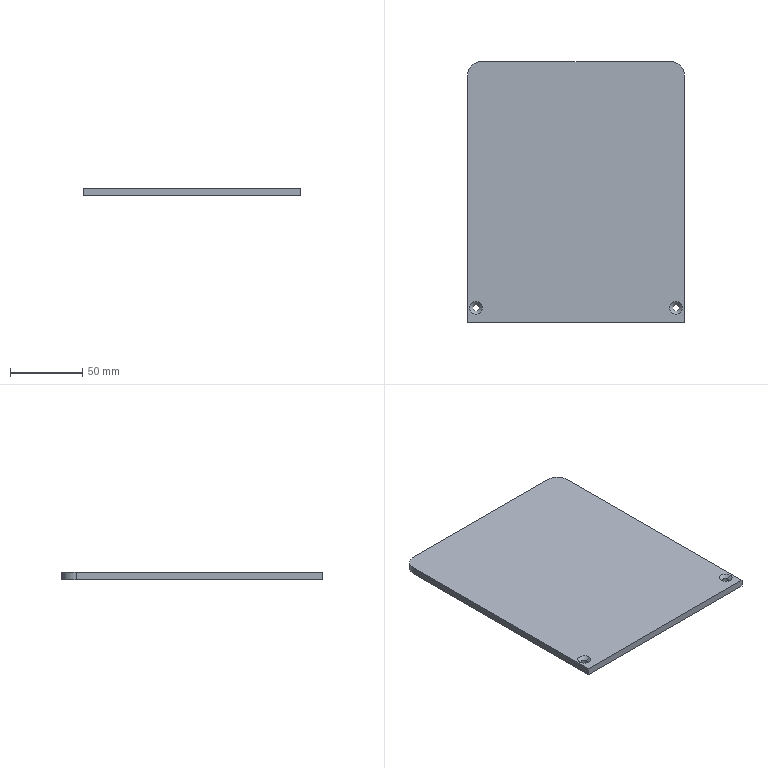Part | STEP file | ND25021-09-JDKM-008-SL | 1 solid | 16 faces | box 150 x 180 x 5 mm | volume 134533 mm3 | cylinder 6 | plane 6 | cone 4 | commonest cylinder face diameters 4.5 x4 20 x2
STEP:
#1=CARTESIAN_POINT('',(0.,0.,0.));
#2=DIRECTION('',(0.,0.,1.));
#3=DIRECTION('',(1.,0.,0.));
#4=AXIS2_PLACEMENT_3D('',#1,#2,#3);
#5=CARTESIAN_POINT('',(71.25,-80.,0.27));
#6=VERTEX_POINT('',#5);
#7=CARTESIAN_POINT('',(73.48,-80.,2.5));
#8=VERTEX_POINT('',#7);
#9=CARTESIAN_POINT('',(73.48,-80.,2.5));
#10=DIRECTION('',(0.7071,0.,0.7071));
#11=VECTOR('',#10,1.);
#12=LINE('',#9,#11);
#13=CARTESIAN_POINT('',(69.,-80.,2.5));
#14=DIRECTION('',(0.,0.,1.));
#15=DIRECTION('',(1.,0.,0.));
#16=AXIS2_PLACEMENT_3D('',#13,#14,#15);
#17=CONICAL_SURFACE('',#16,4.48,0.7854);
#18=CARTESIAN_POINT('',(6.283,0.));
#19=DIRECTION('',(0.,1.));
#20=VECTOR('',#19,1.);
#21=LINE('',#18,#20);
#22=(GEOMETRIC_REPRESENTATION_CONTEXT(2)PARAMETRIC_REPRESENTATION_CONTEXT()REPRESENTATION_CONTEXT('',''));
#23=DEFINITIONAL_REPRESENTATION('',(#21),#22);
#24=PCURVE('',#17,#23);
#25=CARTESIAN_POINT('',(69.,-80.,2.5));
#26=DIRECTION('',(0.,0.,1.));
#27=DIRECTION('',(1.,0.,0.));
#28=AXIS2_PLACEMENT_3D('',#25,#26,#27);
#29=CONICAL_SURFACE('',#28,4.48,0.7854);
#30=CARTESIAN_POINT('',(0.,0.));
#31=DIRECTION('',(0.,1.));
#32=VECTOR('',#31,1.);
#33=LINE('',#30,#32);
#34=(GEOMETRIC_REPRESENTATION_CONTEXT(2)PARAMETRIC_REPRESENTATION_CONTEXT()REPRESENTATION_CONTEXT('',''));
#35=DEFINITIONAL_REPRESENTATION('',(#33),#34);
#36=PCURVE('',#29,#35);
#37=SURFACE_CURVE('',#12,(#24,#36),.PCURVE_S1.);
#38=EDGE_CURVE('',#6,#8,#37,.T.);
#39=ORIENTED_EDGE('',*,*,#38,.T.);
#40=CARTESIAN_POINT('',(64.52,-80.,2.5));
#41=VERTEX_POINT('',#40);
#42=CARTESIAN_POINT('',(69.,-80.,2.5));
#43=DIRECTION('',(0.,0.,1.));
#44=DIRECTION('',(1.,0.,0.));
#45=AXIS2_PLACEMENT_3D('',#42,#43,#44);
#46=CIRCLE('',#45,4.48);
#47=CARTESIAN_POINT('',(0.,0.));
#48=DIRECTION('',(1.,0.));
#49=VECTOR('',#48,1.);
#50=LINE('',#47,#49);
#51=(GEOMETRIC_REPRESENTATION_CONTEXT(2)PARAMETRIC_REPRESENTATION_CONTEXT()REPRESENTATION_CONTEXT('',''));
#52=DEFINITIONAL_REPRESENTATION('',(#50),#51);
#53=PCURVE('',#17,#52);
#54=CARTESIAN_POINT('',(0.,0.,2.5));
#55=DIRECTION('',(0.,0.,1.));
#56=DIRECTION('',(1.,0.,0.));
#57=AXIS2_PLACEMENT_3D('',#54,#55,#56);
#58=PLANE('',#57);
#59=CARTESIAN_POINT('',(69.,-80.));
#60=DIRECTION('',(1.,0.));
#61=AXIS2_PLACEMENT_2D('',#59,#60);
#62=CIRCLE('',#61,4.48);
#63=(GEOMETRIC_REPRESENTATION_CONTEXT(2)PARAMETRIC_REPRESENTATION_CONTEXT()REPRESENTATION_CONTEXT('',''));
#64=DEFINITIONAL_REPRESENTATION('',(#62),#63);
#65=PCURVE('',#58,#64);
#66=SURFACE_CURVE('',#46,(#53,#65),.PCURVE_S1.);
#67=EDGE_CURVE('',#41,#8,#66,.T.);
#68=ORIENTED_EDGE('',*,*,#67,.F.);
#69=CARTESIAN_POINT('',(66.75,-80.,0.27));
#70=VERTEX_POINT('',#69);
#71=CARTESIAN_POINT('',(64.52,-80.,2.5));
#72=DIRECTION('',(-0.7071,0.,0.7071));
#73=VECTOR('',#72,1.);
#74=LINE('',#71,#73);
#75=CARTESIAN_POINT('',(3.142,0.));
#76=DIRECTION('',(0.,1.));
#77=VECTOR('',#76,1.);
#78=LINE('',#75,#77);
#79=(GEOMETRIC_REPRESENTATION_CONTEXT(2)PARAMETRIC_REPRESENTATION_CONTEXT()REPRESENTATION_CONTEXT('',''));
#80=DEFINITIONAL_REPRESENTATION('',(#78),#79);
#81=PCURVE('',#17,#80);
#82=CARTESIAN_POINT('',(3.142,0.));
#83=DIRECTION('',(0.,1.));
#84=VECTOR('',#83,1.);
#85=LINE('',#82,#84);
#86=(GEOMETRIC_REPRESENTATION_CONTEXT(2)PARAMETRIC_REPRESENTATION_CONTEXT()REPRESENTATION_CONTEXT('',''));
#87=DEFINITIONAL_REPRESENTATION('',(#85),#86);
#88=PCURVE('',#29,#87);
#89=SURFACE_CURVE('',#74,(#81,#88),.PCURVE_S1.);
#90=EDGE_CURVE('',#70,#41,#89,.T.);
#91=ORIENTED_EDGE('',*,*,#90,.F.);
#92=CARTESIAN_POINT('',(69.,-80.,0.27));
#93=DIRECTION('',(0.,0.,1.));
#94=DIRECTION('',(1.,0.,0.));
#95=AXIS2_PLACEMENT_3D('',#92,#93,#94);
#96=CIRCLE('',#95,2.25);
#97=CARTESIAN_POINT('',(0.,-2.23));
#98=DIRECTION('',(1.,0.));
#99=VECTOR('',#98,1.);
#100=LINE('',#97,#99);
#101=(GEOMETRIC_REPRESENTATION_CONTEXT(2)PARAMETRIC_REPRESENTATION_CONTEXT()REPRESENTATION_CONTEXT('',''));
#102=DEFINITIONAL_REPRESENTATION('',(#100),#101);
#103=PCURVE('',#17,#102);
#104=CARTESIAN_POINT('',(69.,-80.,2.5));
#105=DIRECTION('',(0.,0.,1.));
#106=DIRECTION('',(1.,0.,0.));
#107=AXIS2_PLACEMENT_3D('',#104,#105,#106);
#108=CYLINDRICAL_SURFACE('',#107,2.25);
#109=CARTESIAN_POINT('',(0.,-2.23));
#110=DIRECTION('',(1.,0.));
#111=VECTOR('',#110,1.);
#112=LINE('',#109,#111);
#113=(GEOMETRIC_REPRESENTATION_CONTEXT(2)PARAMETRIC_REPRESENTATION_CONTEXT()REPRESENTATION_CONTEXT('',''));
#114=DEFINITIONAL_REPRESENTATION('',(#112),#113);
#115=PCURVE('',#108,#114);
#116=SURFACE_CURVE('',#96,(#103,#115),.PCURVE_S1.);
#117=EDGE_CURVE('',#70,#6,#116,.T.);
#118=ORIENTED_EDGE('',*,*,#117,.T.);
#119=EDGE_LOOP('',(#39,#68,#91,#118));
#120=FACE_BOUND('',#119,.F.);
#121=ADVANCED_FACE('',(#120),#17,.F.);
#122=CARTESIAN_POINT('',(71.25,-80.,-2.5));
#123=VERTEX_POINT('',#122);
#124=CARTESIAN_POINT('',(71.25,-80.,2.5));
#125=DIRECTION('',(0.,0.,1.));
#126=VECTOR('',#125,1.);
#127=LINE('',#124,#126);
#128=CARTESIAN_POINT('',(6.283,0.));
#129=DIRECTION('',(0.,1.));
#130=VECTOR('',#129,1.);
#131=LINE('',#128,#130);
#132=(GEOMETRIC_REPRESENTATION_CONTEXT(2)PARAMETRIC_REPRESENTATION_CONTEXT()REPRESENTATION_CONTEXT('',''));
#133=DEFINITIONAL_REPRESENTATION('',(#131),#132);
#134=PCURVE('',#108,#133);
#135=CARTESIAN_POINT('',(69.,-80.,2.5));
#136=DIRECTION('',(0.,0.,1.));
#137=DIRECTION('',(1.,0.,0.));
#138=AXIS2_PLACEMENT_3D('',#135,#136,#137);
#139=CYLINDRICAL_SURFACE('',#138,2.25);
#140=CARTESIAN_POINT('',(0.,0.));
#141=DIRECTION('',(0.,1.));
#142=VECTOR('',#141,1.);
#143=LINE('',#140,#142);
#144=(GEOMETRIC_REPRESENTATION_CONTEXT(2)PARAMETRIC_REPRESENTATION_CONTEXT()REPRESENTATION_CONTEXT('',''));
#145=DEFINITIONAL_REPRESENTATION('',(#143),#144);
#146=PCURVE('',#139,#145);
#147=SURFACE_CURVE('',#127,(#134,#146),.PCURVE_S1.);
#148=EDGE_CURVE('',#123,#6,#147,.T.);
#149=ORIENTED_EDGE('',*,*,#148,.T.);
#150=ORIENTED_EDGE('',*,*,#117,.F.);
#151=CARTESIAN_POINT('',(66.75,-80.,-2.5));
#152=VERTEX_POINT('',#151);
#153=CARTESIAN_POINT('',(66.75,-80.,2.5));
#154=DIRECTION('',(0.,0.,1.));
#155=VECTOR('',#154,1.);
#156=LINE('',#153,#155);
#157=CARTESIAN_POINT('',(3.142,0.));
#158=DIRECTION('',(0.,1.));
#159=VECTOR('',#158,1.);
#160=LINE('',#157,#159);
#161=(GEOMETRIC_REPRESENTATION_CONTEXT(2)PARAMETRIC_REPRESENTATION_CONTEXT()REPRESENTATION_CONTEXT('',''));
#162=DEFINITIONAL_REPRESENTATION('',(#160),#161);
#163=PCURVE('',#108,#162);
#164=CARTESIAN_POINT('',(3.142,0.));
#165=DIRECTION('',(0.,1.));
#166=VECTOR('',#165,1.);
#167=LINE('',#164,#166);
#168=(GEOMETRIC_REPRESENTATION_CONTEXT(2)PARAMETRIC_REPRESENTATION_CONTEXT()REPRESENTATION_CONTEXT('',''));
#169=DEFINITIONAL_REPRESENTATION('',(#167),#168);
#170=PCURVE('',#139,#169);
#171=SURFACE_CURVE('',#156,(#163,#170),.PCURVE_S1.);
#172=EDGE_CURVE('',#152,#70,#171,.T.);
#173=ORIENTED_EDGE('',*,*,#172,.F.);
#174=CARTESIAN_POINT('',(69.,-80.,-2.5));
#175=DIRECTION('',(0.,0.,1.));
#176=DIRECTION('',(1.,0.,0.));
#177=AXIS2_PLACEMENT_3D('',#174,#175,#176);
#178=CIRCLE('',#177,2.25);
#179=CARTESIAN_POINT('',(0.,-5.));
#180=DIRECTION('',(1.,0.));
#181=VECTOR('',#180,1.);
#182=LINE('',#179,#181);
#183=(GEOMETRIC_REPRESENTATION_CONTEXT(2)PARAMETRIC_REPRESENTATION_CONTEXT()REPRESENTATION_CONTEXT('',''));
#184=DEFINITIONAL_REPRESENTATION('',(#182),#183);
#185=PCURVE('',#108,#184);
#186=CARTESIAN_POINT('',(0.,0.,-2.5));
#187=DIRECTION('',(0.,0.,1.));
#188=DIRECTION('',(1.,0.,0.));
#189=AXIS2_PLACEMENT_3D('',#186,#187,#188);
#190=PLANE('',#189);
#191=CARTESIAN_POINT('',(69.,-80.));
#192=DIRECTION('',(1.,0.));
#193=AXIS2_PLACEMENT_2D('',#191,#192);
#194=CIRCLE('',#193,2.25);
#195=(GEOMETRIC_REPRESENTATION_CONTEXT(2)PARAMETRIC_REPRESENTATION_CONTEXT()REPRESENTATION_CONTEXT('',''));
#196=DEFINITIONAL_REPRESENTATION('',(#194),#195);
#197=PCURVE('',#190,#196);
#198=SURFACE_CURVE('',#178,(#185,#197),.PCURVE_S1.);
#199=EDGE_CURVE('',#152,#123,#198,.T.);
#200=ORIENTED_EDGE('',*,*,#199,.T.);
#201=EDGE_LOOP('',(#149,#150,#173,#200));
#202=FACE_BOUND('',#201,.F.);
#203=ADVANCED_FACE('',(#202),#108,.F.);
#204=CARTESIAN_POINT('',(-66.75,-80.,0.27));
#205=VERTEX_POINT('',#204);
#206=CARTESIAN_POINT('',(-64.52,-80.,2.5));
#207=VERTEX_POINT('',#206);
#208=CARTESIAN_POINT('',(-64.52,-80.,2.5));
#209=DIRECTION('',(0.7071,0.,0.7071));
#210=VECTOR('',#209,1.);
#211=LINE('',#208,#210);
#212=CARTESIAN_POINT('',(-69.,-80.,2.5));
#213=DIRECTION('',(0.,0.,1.));
#214=DIRECTION('',(1.,0.,0.));
#215=AXIS2_PLACEMENT_3D('',#212,#213,#214);
#216=CONICAL_SURFACE('',#215,4.48,0.7854);
#217=CARTESIAN_POINT('',(6.283,0.));
#218=DIRECTION('',(0.,1.));
#219=VECTOR('',#218,1.);
#220=LINE('',#217,#219);
#221=(GEOMETRIC_REPRESENTATION_CONTEXT(2)PARAMETRIC_REPRESENTATION_CONTEXT()REPRESENTATION_CONTEXT('',''));
#222=DEFINITIONAL_REPRESENTATION('',(#220),#221);
#223=PCURVE('',#216,#222);
#224=CARTESIAN_POINT('',(-69.,-80.,2.5));
#225=DIRECTION('',(0.,0.,1.));
#226=DIRECTION('',(1.,0.,0.));
#227=AXIS2_PLACEMENT_3D('',#224,#225,#226);
#228=CONICAL_SURFACE('',#227,4.48,0.7854);
#229=CARTESIAN_POINT('',(0.,0.));
#230=DIRECTION('',(0.,1.));
#231=VECTOR('',#230,1.);
#232=LINE('',#229,#231);
#233=(GEOMETRIC_REPRESENTATION_CONTEXT(2)PARAMETRIC_REPRESENTATION_CONTEXT()REPRESENTATION_CONTEXT('',''));
#234=DEFINITIONAL_REPRESENTATION('',(#232),#233);
#235=PCURVE('',#228,#234);
#236=SURFACE_CURVE('',#211,(#223,#235),.PCURVE_S1.);
#237=EDGE_CURVE('',#205,#207,#236,.T.);
#238=ORIENTED_EDGE('',*,*,#237,.T.);
#239=CARTESIAN_POINT('',(-73.48,-80.,2.5));
#240=VERTEX_POINT('',#239);
#241=CARTESIAN_POINT('',(-69.,-80.,2.5));
#242=DIRECTION('',(0.,0.,1.));
#243=DIRECTION('',(1.,0.,0.));
#244=AXIS2_PLACEMENT_3D('',#241,#242,#243);
#245=CIRCLE('',#244,4.48);
#246=CARTESIAN_POINT('',(0.,0.));
#247=DIRECTION('',(1.,0.));
#248=VECTOR('',#247,1.);
#249=LINE('',#246,#248);
#250=(GEOMETRIC_REPRESENTATION_CONTEXT(2)PARAMETRIC_REPRESENTATION_CONTEXT()REPRESENTATION_CONTEXT('',''));
#251=DEFINITIONAL_REPRESENTATION('',(#249),#250);
#252=PCURVE('',#216,#251);
#253=CARTESIAN_POINT('',(-69.,-80.));
#254=DIRECTION('',(1.,0.));
#255=AXIS2_PLACEMENT_2D('',#253,#254);
#256=CIRCLE('',#255,4.48);
#257=(GEOMETRIC_REPRESENTATION_CONTEXT(2)PARAMETRIC_REPRESENTATION_CONTEXT()REPRESENTATION_CONTEXT('',''));
#258=DEFINITIONAL_REPRESENTATION('',(#256),#257);
#259=PCURVE('',#58,#258);
#260=SURFACE_CURVE('',#245,(#252,#259),.PCURVE_S1.);
#261=EDGE_CURVE('',#240,#207,#260,.T.);
#262=ORIENTED_EDGE('',*,*,#261,.F.);
#263=CARTESIAN_POINT('',(-71.25,-80.,0.27));
#264=VERTEX_POINT('',#263);
#265=CARTESIAN_POINT('',(-73.48,-80.,2.5));
#266=DIRECTION('',(-0.7071,0.,0.7071));
#267=VECTOR('',#266,1.);
#268=LINE('',#265,#267);
#269=CARTESIAN_POINT('',(3.142,0.));
#270=DIRECTION('',(0.,1.));
#271=VECTOR('',#270,1.);
#272=LINE('',#269,#271);
#273=(GEOMETRIC_REPRESENTATION_CONTEXT(2)PARAMETRIC_REPRESENTATION_CONTEXT()REPRESENTATION_CONTEXT('',''));
#274=DEFINITIONAL_REPRESENTATION('',(#272),#273);
#275=PCURVE('',#216,#274);
#276=CARTESIAN_POINT('',(3.142,0.));
#277=DIRECTION('',(0.,1.));
#278=VECTOR('',#277,1.);
#279=LINE('',#276,#278);
#280=(GEOMETRIC_REPRESENTATION_CONTEXT(2)PARAMETRIC_REPRESENTATION_CONTEXT()REPRESENTATION_CONTEXT('',''));
#281=DEFINITIONAL_REPRESENTATION('',(#279),#280);
#282=PCURVE('',#228,#281);
#283=SURFACE_CURVE('',#268,(#275,#282),.PCURVE_S1.);
#284=EDGE_CURVE('',#264,#240,#283,.T.);
#285=ORIENTED_EDGE('',*,*,#284,.F.);
#286=CARTESIAN_POINT('',(-69.,-80.,0.27));
#287=DIRECTION('',(0.,0.,1.));
#288=DIRECTION('',(1.,0.,0.));
#289=AXIS2_PLACEMENT_3D('',#286,#287,#288);
#290=CIRCLE('',#289,2.25);
#291=CARTESIAN_POINT('',(0.,-2.23));
#292=DIRECTION('',(1.,0.));
#293=VECTOR('',#292,1.);
#294=LINE('',#291,#293);
#295=(GEOMETRIC_REPRESENTATION_CONTEXT(2)PARAMETRIC_REPRESENTATION_CONTEXT()REPRESENTATION_CONTEXT('',''));
#296=DEFINITIONAL_REPRESENTATION('',(#294),#295);
#297=PCURVE('',#216,#296);
#298=CARTESIAN_POINT('',(-69.,-80.,2.5));
#299=DIRECTION('',(0.,0.,1.));
#300=DIRECTION('',(1.,0.,0.));
#301=AXIS2_PLACEMENT_3D('',#298,#299,#300);
#302=CYLINDRICAL_SURFACE('',#301,2.25);
#303=CARTESIAN_POINT('',(0.,-2.23));
#304=DIRECTION('',(1.,0.));
#305=VECTOR('',#304,1.);
#306=LINE('',#303,#305);
#307=(GEOMETRIC_REPRESENTATION_CONTEXT(2)PARAMETRIC_REPRESENTATION_CONTEXT()REPRESENTATION_CONTEXT('',''));
#308=DEFINITIONAL_REPRESENTATION('',(#306),#307);
#309=PCURVE('',#302,#308);
#310=SURFACE_CURVE('',#290,(#297,#309),.PCURVE_S1.);
#311=EDGE_CURVE('',#264,#205,#310,.T.);
#312=ORIENTED_EDGE('',*,*,#311,.T.);
#313=EDGE_LOOP('',(#238,#262,#285,#312));
#314=FACE_BOUND('',#313,.F.);
#315=ADVANCED_FACE('',(#314),#216,.F.);
#316=CARTESIAN_POINT('',(-66.75,-80.,-2.5));
#317=VERTEX_POINT('',#316);
#318=CARTESIAN_POINT('',(-66.75,-80.,2.5));
#319=DIRECTION('',(0.,0.,1.));
#320=VECTOR('',#319,1.);
#321=LINE('',#318,#320);
#322=CARTESIAN_POINT('',(6.283,0.));
#323=DIRECTION('',(0.,1.));
#324=VECTOR('',#323,1.);
#325=LINE('',#322,#324);
#326=(GEOMETRIC_REPRESENTATION_CONTEXT(2)PARAMETRIC_REPRESENTATION_CONTEXT()REPRESENTATION_CONTEXT('',''));
#327=DEFINITIONAL_REPRESENTATION('',(#325),#326);
#328=PCURVE('',#302,#327);
#329=CARTESIAN_POINT('',(-69.,-80.,2.5));
#330=DIRECTION('',(0.,0.,1.));
#331=DIRECTION('',(1.,0.,0.));
#332=AXIS2_PLACEMENT_3D('',#329,#330,#331);
#333=CYLINDRICAL_SURFACE('',#332,2.25);
#334=CARTESIAN_POINT('',(0.,0.));
#335=DIRECTION('',(0.,1.));
#336=VECTOR('',#335,1.);
#337=LINE('',#334,#336);
#338=(GEOMETRIC_REPRESENTATION_CONTEXT(2)PARAMETRIC_REPRESENTATION_CONTEXT()REPRESENTATION_CONTEXT('',''));
#339=DEFINITIONAL_REPRESENTATION('',(#337),#338);
#340=PCURVE('',#333,#339);
#341=SURFACE_CURVE('',#321,(#328,#340),.PCURVE_S1.);
#342=EDGE_CURVE('',#317,#205,#341,.T.);
#343=ORIENTED_EDGE('',*,*,#342,.T.);
#344=ORIENTED_EDGE('',*,*,#311,.F.);
#345=CARTESIAN_POINT('',(-71.25,-80.,-2.5));
#346=VERTEX_POINT('',#345);
#347=CARTESIAN_POINT('',(-71.25,-80.,2.5));
#348=DIRECTION('',(0.,0.,1.));
#349=VECTOR('',#348,1.);
#350=LINE('',#347,#349);
#351=CARTESIAN_POINT('',(3.142,0.));
#352=DIRECTION('',(0.,1.));
#353=VECTOR('',#352,1.);
#354=LINE('',#351,#353);
#355=(GEOMETRIC_REPRESENTATION_CONTEXT(2)PARAMETRIC_REPRESENTATION_CONTEXT()REPRESENTATION_CONTEXT('',''));
#356=DEFINITIONAL_REPRESENTATION('',(#354),#355);
#357=PCURVE('',#302,#356);
#358=CARTESIAN_POINT('',(3.142,0.));
#359=DIRECTION('',(0.,1.));
#360=VECTOR('',#359,1.);
#361=LINE('',#358,#360);
#362=(GEOMETRIC_REPRESENTATION_CONTEXT(2)PARAMETRIC_REPRESENTATION_CONTEXT()REPRESENTATION_CONTEXT('',''));
#363=DEFINITIONAL_REPRESENTATION('',(#361),#362);
#364=PCURVE('',#333,#363);
#365=SURFACE_CURVE('',#350,(#357,#364),.PCURVE_S1.);
#366=EDGE_CURVE('',#346,#264,#365,.T.);
#367=ORIENTED_EDGE('',*,*,#366,.F.);
#368=CARTESIAN_POINT('',(-69.,-80.,-2.5));
#369=DIRECTION('',(0.,0.,1.));
#370=DIRECTION('',(1.,0.,0.));
#371=AXIS2_PLACEMENT_3D('',#368,#369,#370);
#372=CIRCLE('',#371,2.25);
#373=CARTESIAN_POINT('',(0.,-5.));
#374=DIRECTION('',(1.,0.));
#375=VECTOR('',#374,1.);
#376=LINE('',#373,#375);
#377=(GEOMETRIC_REPRESENTATION_CONTEXT(2)PARAMETRIC_REPRESENTATION_CONTEXT()REPRESENTATION_CONTEXT('',''));
#378=DEFINITIONAL_REPRESENTATION('',(#376),#377);
#379=PCURVE('',#302,#378);
#380=CARTESIAN_POINT('',(-69.,-80.));
#381=DIRECTION('',(1.,0.));
#382=AXIS2_PLACEMENT_2D('',#380,#381);
#383=CIRCLE('',#382,2.25);
#384=(GEOMETRIC_REPRESENTATION_CONTEXT(2)PARAMETRIC_REPRESENTATION_CONTEXT()REPRESENTATION_CONTEXT('',''));
#385=DEFINITIONAL_REPRESENTATION('',(#383),#384);
#386=PCURVE('',#190,#385);
#387=SURFACE_CURVE('',#372,(#379,#386),.PCURVE_S1.);
#388=EDGE_CURVE('',#346,#317,#387,.T.);
#389=ORIENTED_EDGE('',*,*,#388,.T.);
#390=EDGE_LOOP('',(#343,#344,#367,#389));
#391=FACE_BOUND('',#390,.F.);
#392=ADVANCED_FACE('',(#391),#302,.F.);
#393=CARTESIAN_POINT('',(75.,-90.,-2.5));
#394=VERTEX_POINT('',#393);
#395=CARTESIAN_POINT('',(75.,80.,-2.5));
#396=VERTEX_POINT('',#395);
#397=CARTESIAN_POINT('',(75.,90.,-2.5));
#398=DIRECTION('',(0.,1.,0.));
#399=VECTOR('',#398,1.);
#400=LINE('',#397,#399);
#401=CARTESIAN_POINT('',(75.,90.,2.5));
#402=DIRECTION('',(-1.,0.,0.));
#403=DIRECTION('',(0.,-1.,0.));
#404=AXIS2_PLACEMENT_3D('',#401,#402,#403);
#405=PLANE('',#404);
#406=CARTESIAN_POINT('',(0.,-5.));
#407=DIRECTION('',(-1.,0.));
#408=VECTOR('',#407,1.);
#409=LINE('',#406,#408);
#410=(GEOMETRIC_REPRESENTATION_CONTEXT(2)PARAMETRIC_REPRESENTATION_CONTEXT()REPRESENTATION_CONTEXT('',''));
#411=DEFINITIONAL_REPRESENTATION('',(#409),#410);
#412=PCURVE('',#405,#411);
#413=CARTESIAN_POINT('',(75.,90.));
#414=DIRECTION('',(0.,1.));
#415=VECTOR('',#414,1.);
#416=LINE('',#413,#415);
#417=(GEOMETRIC_REPRESENTATION_CONTEXT(2)PARAMETRIC_REPRESENTATION_CONTEXT()REPRESENTATION_CONTEXT('',''));
#418=DEFINITIONAL_REPRESENTATION('',(#416),#417);
#419=PCURVE('',#190,#418);
#420=SURFACE_CURVE('',#400,(#412,#419),.PCURVE_S1.);
#421=EDGE_CURVE('',#394,#396,#420,.T.);
#422=ORIENTED_EDGE('',*,*,#421,.T.);
#423=CARTESIAN_POINT('',(75.,80.,2.5));
#424=VERTEX_POINT('',#423);
#425=CARTESIAN_POINT('',(75.,80.,2.5));
#426=DIRECTION('',(0.,0.,1.));
#427=VECTOR('',#426,1.);
#428=LINE('',#425,#427);
#429=CARTESIAN_POINT('',(10.,0.));
#430=DIRECTION('',(0.,1.));
#431=VECTOR('',#430,1.);
#432=LINE('',#429,#431);
#433=(GEOMETRIC_REPRESENTATION_CONTEXT(2)PARAMETRIC_REPRESENTATION_CONTEXT()REPRESENTATION_CONTEXT('',''));
#434=DEFINITIONAL_REPRESENTATION('',(#432),#433);
#435=PCURVE('',#405,#434);
#436=CARTESIAN_POINT('',(65.,80.,2.5));
#437=DIRECTION('',(0.,0.,-1.));
#438=DIRECTION('',(-1.,0.,0.));
#439=AXIS2_PLACEMENT_3D('',#436,#437,#438);
#440=CYLINDRICAL_SURFACE('',#439,10.);
#441=CARTESIAN_POINT('',(3.142,0.));
#442=DIRECTION('',(0.,-1.));
#443=VECTOR('',#442,1.);
#444=LINE('',#441,#443);
#445=(GEOMETRIC_REPRESENTATION_CONTEXT(2)PARAMETRIC_REPRESENTATION_CONTEXT()REPRESENTATION_CONTEXT('',''));
#446=DEFINITIONAL_REPRESENTATION('',(#444),#445);
#447=PCURVE('',#440,#446);
#448=SURFACE_CURVE('',#428,(#435,#447),.PCURVE_S1.);
#449=EDGE_CURVE('',#396,#424,#448,.T.);
#450=ORIENTED_EDGE('',*,*,#449,.T.);
#451=CARTESIAN_POINT('',(75.,-90.,2.5));
#452=VERTEX_POINT('',#451);
#453=CARTESIAN_POINT('',(75.,90.,2.5));
#454=DIRECTION('',(0.,1.,0.));
#455=VECTOR('',#454,1.);
#456=LINE('',#453,#455);
#457=CARTESIAN_POINT('',(0.,0.));
#458=DIRECTION('',(-1.,0.));
#459=VECTOR('',#458,1.);
#460=LINE('',#457,#459);
#461=(GEOMETRIC_REPRESENTATION_CONTEXT(2)PARAMETRIC_REPRESENTATION_CONTEXT()REPRESENTATION_CONTEXT('',''));
#462=DEFINITIONAL_REPRESENTATION('',(#460),#461);
#463=PCURVE('',#405,#462);
#464=CARTESIAN_POINT('',(75.,90.));
#465=DIRECTION('',(0.,1.));
#466=VECTOR('',#465,1.);
#467=LINE('',#464,#466);
#468=(GEOMETRIC_REPRESENTATION_CONTEXT(2)PARAMETRIC_REPRESENTATION_CONTEXT()REPRESENTATION_CONTEXT('',''));
#469=DEFINITIONAL_REPRESENTATION('',(#467),#468);
#470=PCURVE('',#58,#469);
#471=SURFACE_CURVE('',#456,(#463,#470),.PCURVE_S1.);
#472=EDGE_CURVE('',#452,#424,#471,.T.);
#473=ORIENTED_EDGE('',*,*,#472,.F.);
#474=CARTESIAN_POINT('',(75.,-90.,2.5));
#475=DIRECTION('',(0.,0.,-1.));
#476=VECTOR('',#475,1.);
#477=LINE('',#474,#476);
#478=CARTESIAN_POINT('',(180.,0.));
#479=DIRECTION('',(0.,-1.));
#480=VECTOR('',#479,1.);
#481=LINE('',#478,#480);
#482=(GEOMETRIC_REPRESENTATION_CONTEXT(2)PARAMETRIC_REPRESENTATION_CONTEXT()REPRESENTATION_CONTEXT('',''));
#483=DEFINITIONAL_REPRESENTATION('',(#481),#482);
#484=PCURVE('',#405,#483);
#485=CARTESIAN_POINT('',(-75.,-90.,2.5));
#486=DIRECTION('',(0.,1.,0.));
#487=DIRECTION('',(0.,0.,1.));
#488=AXIS2_PLACEMENT_3D('',#485,#486,#487);
#489=PLANE('',#488);
#490=CARTESIAN_POINT('',(0.,150.));
#491=DIRECTION('',(-1.,0.));
#492=VECTOR('',#491,1.);
#493=LINE('',#490,#492);
#494=(GEOMETRIC_REPRESENTATION_CONTEXT(2)PARAMETRIC_REPRESENTATION_CONTEXT()REPRESENTATION_CONTEXT('',''));
#495=DEFINITIONAL_REPRESENTATION('',(#493),#494);
#496=PCURVE('',#489,#495);
#497=SURFACE_CURVE('',#477,(#484,#496),.PCURVE_S1.);
#498=EDGE_CURVE('',#452,#394,#497,.T.);
#499=ORIENTED_EDGE('',*,*,#498,.T.);
#500=EDGE_LOOP('',(#422,#450,#473,#499));
#501=FACE_BOUND('',#500,.T.);
#502=ADVANCED_FACE('',(#501),#405,.F.);
#503=CARTESIAN_POINT('',(65.,90.,-2.5));
#504=VERTEX_POINT('',#503);
#505=CARTESIAN_POINT('',(-65.,90.,-2.5));
#506=VERTEX_POINT('',#505);
#507=CARTESIAN_POINT('',(-75.,90.,-2.5));
#508=DIRECTION('',(-1.,0.,0.));
#509=VECTOR('',#508,1.);
#510=LINE('',#507,#509);
#511=CARTESIAN_POINT('',(-75.,90.,2.5));
#512=DIRECTION('',(0.,-1.,0.));
#513=DIRECTION('',(0.,0.,-1.));
#514=AXIS2_PLACEMENT_3D('',#511,#512,#513);
#515=PLANE('',#514);
#516=CARTESIAN_POINT('',(5.,0.));
#517=DIRECTION('',(0.,-1.));
#518=VECTOR('',#517,1.);
#519=LINE('',#516,#518);
#520=(GEOMETRIC_REPRESENTATION_CONTEXT(2)PARAMETRIC_REPRESENTATION_CONTEXT()REPRESENTATION_CONTEXT('',''));
#521=DEFINITIONAL_REPRESENTATION('',(#519),#520);
#522=PCURVE('',#515,#521);
#523=CARTESIAN_POINT('',(-75.,90.));
#524=DIRECTION('',(-1.,0.));
#525=VECTOR('',#524,1.);
#526=LINE('',#523,#525);
#527=(GEOMETRIC_REPRESENTATION_CONTEXT(2)PARAMETRIC_REPRESENTATION_CONTEXT()REPRESENTATION_CONTEXT('',''));
#528=DEFINITIONAL_REPRESENTATION('',(#526),#527);
#529=PCURVE('',#190,#528);
#530=SURFACE_CURVE('',#510,(#522,#529),.PCURVE_S1.);
#531=EDGE_CURVE('',#504,#506,#530,.T.);
#532=ORIENTED_EDGE('',*,*,#531,.T.);
#533=CARTESIAN_POINT('',(-65.,90.,2.5));
#534=VERTEX_POINT('',#533);
#535=CARTESIAN_POINT('',(-65.,90.,2.5));
#536=DIRECTION('',(0.,0.,1.));
#537=VECTOR('',#536,1.);
#538=LINE('',#535,#537);
#539=CARTESIAN_POINT('',(0.,10.));
#540=DIRECTION('',(-1.,0.));
#541=VECTOR('',#540,1.);
#542=LINE('',#539,#541);
#543=(GEOMETRIC_REPRESENTATION_CONTEXT(2)PARAMETRIC_REPRESENTATION_CONTEXT()REPRESENTATION_CONTEXT('',''));
#544=DEFINITIONAL_REPRESENTATION('',(#542),#543);
#545=PCURVE('',#515,#544);
#546=CARTESIAN_POINT('',(-65.,80.,2.5));
#547=DIRECTION('',(0.,0.,-1.));
#548=DIRECTION('',(-1.,0.,0.));
#549=AXIS2_PLACEMENT_3D('',#546,#547,#548);
#550=CYLINDRICAL_SURFACE('',#549,10.);
#551=CARTESIAN_POINT('',(1.571,0.));
#552=DIRECTION('',(0.,-1.));
#553=VECTOR('',#552,1.);
#554=LINE('',#551,#553);
#555=(GEOMETRIC_REPRESENTATION_CONTEXT(2)PARAMETRIC_REPRESENTATION_CONTEXT()REPRESENTATION_CONTEXT('',''));
#556=DEFINITIONAL_REPRESENTATION('',(#554),#555);
#557=PCURVE('',#550,#556);
#558=SURFACE_CURVE('',#538,(#545,#557),.PCURVE_S1.);
#559=EDGE_CURVE('',#506,#534,#558,.T.);
#560=ORIENTED_EDGE('',*,*,#559,.T.);
#561=CARTESIAN_POINT('',(65.,90.,2.5));
#562=VERTEX_POINT('',#561);
#563=CARTESIAN_POINT('',(-75.,90.,2.5));
#564=DIRECTION('',(-1.,0.,0.));
#565=VECTOR('',#564,1.);
#566=LINE('',#563,#565);
#567=CARTESIAN_POINT('',(0.,0.));
#568=DIRECTION('',(0.,-1.));
#569=VECTOR('',#568,1.);
#570=LINE('',#567,#569);
#571=(GEOMETRIC_REPRESENTATION_CONTEXT(2)PARAMETRIC_REPRESENTATION_CONTEXT()REPRESENTATION_CONTEXT('',''));
#572=DEFINITIONAL_REPRESENTATION('',(#570),#571);
#573=PCURVE('',#515,#572);
#574=CARTESIAN_POINT('',(-75.,90.));
#575=DIRECTION('',(-1.,0.));
#576=VECTOR('',#575,1.);
#577=LINE('',#574,#576);
#578=(GEOMETRIC_REPRESENTATION_CONTEXT(2)PARAMETRIC_REPRESENTATION_CONTEXT()REPRESENTATION_CONTEXT('',''));
#579=DEFINITIONAL_REPRESENTATION('',(#577),#578);
#580=PCURVE('',#58,#579);
#581=SURFACE_CURVE('',#566,(#573,#580),.PCURVE_S1.);
#582=EDGE_CURVE('',#562,#534,#581,.T.);
#583=ORIENTED_EDGE('',*,*,#582,.F.);
#584=CARTESIAN_POINT('',(65.,90.,2.5));
#585=DIRECTION('',(0.,0.,-1.));
#586=VECTOR('',#585,1.);
#587=LINE('',#584,#586);
#588=CARTESIAN_POINT('',(0.,140.));
#589=DIRECTION('',(1.,0.));
#590=VECTOR('',#589,1.);
#591=LINE('',#588,#590);
#592=(GEOMETRIC_REPRESENTATION_CONTEXT(2)PARAMETRIC_REPRESENTATION_CONTEXT()REPRESENTATION_CONTEXT('',''));
#593=DEFINITIONAL_REPRESENTATION('',(#591),#592);
#594=PCURVE('',#515,#593);
#595=CARTESIAN_POINT('',(1.571,0.));
#596=DIRECTION('',(0.,1.));
#597=VECTOR('',#596,1.);
#598=LINE('',#595,#597);
#599=(GEOMETRIC_REPRESENTATION_CONTEXT(2)PARAMETRIC_REPRESENTATION_CONTEXT()REPRESENTATION_CONTEXT('',''));
#600=DEFINITIONAL_REPRESENTATION('',(#598),#599);
#601=PCURVE('',#440,#600);
#602=SURFACE_CURVE('',#587,(#594,#601),.PCURVE_S1.);
#603=EDGE_CURVE('',#562,#504,#602,.T.);
#604=ORIENTED_EDGE('',*,*,#603,.T.);
#605=EDGE_LOOP('',(#532,#560,#583,#604));
#606=FACE_BOUND('',#605,.T.);
#607=ADVANCED_FACE('',(#606),#515,.F.);
#608=CARTESIAN_POINT('',(-75.,80.,2.5));
#609=VERTEX_POINT('',#608);
#610=CARTESIAN_POINT('',(-75.,-90.,2.5));
#611=VERTEX_POINT('',#610);
#612=CARTESIAN_POINT('',(-75.,90.,2.5));
#613=DIRECTION('',(0.,-1.,0.));
#614=VECTOR('',#613,1.);
#615=LINE('',#612,#614);
#616=CARTESIAN_POINT('',(-75.,90.,2.5));
#617=DIRECTION('',(1.,0.,0.));
#618=DIRECTION('',(0.,1.,0.));
#619=AXIS2_PLACEMENT_3D('',#616,#617,#618);
#620=PLANE('',#619);
#621=CARTESIAN_POINT('',(0.,0.));
#622=DIRECTION('',(-1.,0.));
#623=VECTOR('',#622,1.);
#624=LINE('',#621,#623);
#625=(GEOMETRIC_REPRESENTATION_CONTEXT(2)PARAMETRIC_REPRESENTATION_CONTEXT()REPRESENTATION_CONTEXT('',''));
#626=DEFINITIONAL_REPRESENTATION('',(#624),#625);
#627=PCURVE('',#620,#626);
#628=CARTESIAN_POINT('',(-75.,90.));
#629=DIRECTION('',(0.,-1.));
#630=VECTOR('',#629,1.);
#631=LINE('',#628,#630);
#632=(GEOMETRIC_REPRESENTATION_CONTEXT(2)PARAMETRIC_REPRESENTATION_CONTEXT()REPRESENTATION_CONTEXT('',''));
#633=DEFINITIONAL_REPRESENTATION('',(#631),#632);
#634=PCURVE('',#58,#633);
#635=SURFACE_CURVE('',#615,(#627,#634),.PCURVE_S1.);
#636=EDGE_CURVE('',#609,#611,#635,.T.);
#637=ORIENTED_EDGE('',*,*,#636,.F.);
#638=CARTESIAN_POINT('',(-75.,80.,-2.5));
#639=VERTEX_POINT('',#638);
#640=CARTESIAN_POINT('',(-75.,80.,2.5));
#641=DIRECTION('',(0.,0.,-1.));
#642=VECTOR('',#641,1.);
#643=LINE('',#640,#642);
#644=CARTESIAN_POINT('',(-10.,0.));
#645=DIRECTION('',(0.,-1.));
#646=VECTOR('',#645,1.);
#647=LINE('',#644,#646);
#648=(GEOMETRIC_REPRESENTATION_CONTEXT(2)PARAMETRIC_REPRESENTATION_CONTEXT()REPRESENTATION_CONTEXT('',''));
#649=DEFINITIONAL_REPRESENTATION('',(#647),#648);
#650=PCURVE('',#620,#649);
#651=CARTESIAN_POINT('',(0.,0.));
#652=DIRECTION('',(0.,1.));
#653=VECTOR('',#652,1.);
#654=LINE('',#651,#653);
#655=(GEOMETRIC_REPRESENTATION_CONTEXT(2)PARAMETRIC_REPRESENTATION_CONTEXT()REPRESENTATION_CONTEXT('',''));
#656=DEFINITIONAL_REPRESENTATION('',(#654),#655);
#657=PCURVE('',#550,#656);
#658=SURFACE_CURVE('',#643,(#650,#657),.PCURVE_S1.);
#659=EDGE_CURVE('',#609,#639,#658,.T.);
#660=ORIENTED_EDGE('',*,*,#659,.T.);
#661=CARTESIAN_POINT('',(-75.,-90.,-2.5));
#662=VERTEX_POINT('',#661);
#663=CARTESIAN_POINT('',(-75.,90.,-2.5));
#664=DIRECTION('',(0.,-1.,0.));
#665=VECTOR('',#664,1.);
#666=LINE('',#663,#665);
#667=CARTESIAN_POINT('',(0.,-5.));
#668=DIRECTION('',(-1.,0.));
#669=VECTOR('',#668,1.);
#670=LINE('',#667,#669);
#671=(GEOMETRIC_REPRESENTATION_CONTEXT(2)PARAMETRIC_REPRESENTATION_CONTEXT()REPRESENTATION_CONTEXT('',''));
#672=DEFINITIONAL_REPRESENTATION('',(#670),#671);
#673=PCURVE('',#620,#672);
#674=CARTESIAN_POINT('',(-75.,90.));
#675=DIRECTION('',(0.,-1.));
#676=VECTOR('',#675,1.);
#677=LINE('',#674,#676);
#678=(GEOMETRIC_REPRESENTATION_CONTEXT(2)PARAMETRIC_REPRESENTATION_CONTEXT()REPRESENTATION_CONTEXT('',''));
#679=DEFINITIONAL_REPRESENTATION('',(#677),#678);
#680=PCURVE('',#190,#679);
#681=SURFACE_CURVE('',#666,(#673,#680),.PCURVE_S1.);
#682=EDGE_CURVE('',#639,#662,#681,.T.);
#683=ORIENTED_EDGE('',*,*,#682,.T.);
#684=CARTESIAN_POINT('',(-75.,-90.,2.5));
#685=DIRECTION('',(0.,0.,-1.));
#686=VECTOR('',#685,1.);
#687=LINE('',#684,#686);
#688=CARTESIAN_POINT('',(-180.,0.));
#689=DIRECTION('',(0.,-1.));
#690=VECTOR('',#689,1.);
#691=LINE('',#688,#690);
#692=(GEOMETRIC_REPRESENTATION_CONTEXT(2)PARAMETRIC_REPRESENTATION_CONTEXT()REPRESENTATION_CONTEXT('',''));
#693=DEFINITIONAL_REPRESENTATION('',(#691),#692);
#694=PCURVE('',#620,#693);
#695=CARTESIAN_POINT('',(0.,0.));
#696=DIRECTION('',(-1.,0.));
#697=VECTOR('',#696,1.);
#698=LINE('',#695,#697);
#699=(GEOMETRIC_REPRESENTATION_CONTEXT(2)PARAMETRIC_REPRESENTATION_CONTEXT()REPRESENTATION_CONTEXT('',''));
#700=DEFINITIONAL_REPRESENTATION('',(#698),#699);
#701=PCURVE('',#489,#700);
#702=SURFACE_CURVE('',#687,(#694,#701),.PCURVE_S1.);
#703=EDGE_CURVE('',#611,#662,#702,.T.);
#704=ORIENTED_EDGE('',*,*,#703,.F.);
#705=EDGE_LOOP('',(#637,#660,#683,#704));
#706=FACE_BOUND('',#705,.T.);
#707=ADVANCED_FACE('',(#706),#620,.F.);
#708=CARTESIAN_POINT('',(-75.,-90.,-2.5));
#709=DIRECTION('',(1.,0.,0.));
#710=VECTOR('',#709,1.);
#711=LINE('',#708,#710);
#712=CARTESIAN_POINT('',(-5.,0.));
#713=DIRECTION('',(0.,1.));
#714=VECTOR('',#713,1.);
#715=LINE('',#712,#714);
#716=(GEOMETRIC_REPRESENTATION_CONTEXT(2)PARAMETRIC_REPRESENTATION_CONTEXT()REPRESENTATION_CONTEXT('',''));
#717=DEFINITIONAL_REPRESENTATION('',(#715),#716);
#718=PCURVE('',#489,#717);
#719=CARTESIAN_POINT('',(-75.,-90.));
#720=DIRECTION('',(1.,0.));
#721=VECTOR('',#720,1.);
#722=LINE('',#719,#721);
#723=(GEOMETRIC_REPRESENTATION_CONTEXT(2)PARAMETRIC_REPRESENTATION_CONTEXT()REPRESENTATION_CONTEXT('',''));
#724=DEFINITIONAL_REPRESENTATION('',(#722),#723);
#725=PCURVE('',#190,#724);
#726=SURFACE_CURVE('',#711,(#718,#725),.PCURVE_S1.);
#727=EDGE_CURVE('',#662,#394,#726,.T.);
#728=ORIENTED_EDGE('',*,*,#727,.T.);
#729=ORIENTED_EDGE('',*,*,#498,.F.);
#730=CARTESIAN_POINT('',(-75.,-90.,2.5));
#731=DIRECTION('',(1.,0.,0.));
#732=VECTOR('',#731,1.);
#733=LINE('',#730,#732);
#734=CARTESIAN_POINT('',(0.,0.));
#735=DIRECTION('',(0.,1.));
#736=VECTOR('',#735,1.);
#737=LINE('',#734,#736);
#738=(GEOMETRIC_REPRESENTATION_CONTEXT(2)PARAMETRIC_REPRESENTATION_CONTEXT()REPRESENTATION_CONTEXT('',''));
#739=DEFINITIONAL_REPRESENTATION('',(#737),#738);
#740=PCURVE('',#489,#739);
#741=CARTESIAN_POINT('',(-75.,-90.));
#742=DIRECTION('',(1.,0.));
#743=VECTOR('',#742,1.);
#744=LINE('',#741,#743);
#745=(GEOMETRIC_REPRESENTATION_CONTEXT(2)PARAMETRIC_REPRESENTATION_CONTEXT()REPRESENTATION_CONTEXT('',''));
#746=DEFINITIONAL_REPRESENTATION('',(#744),#745);
#747=PCURVE('',#58,#746);
#748=SURFACE_CURVE('',#733,(#740,#747),.PCURVE_S1.);
#749=EDGE_CURVE('',#611,#452,#748,.T.);
#750=ORIENTED_EDGE('',*,*,#749,.F.);
#751=ORIENTED_EDGE('',*,*,#703,.T.);
#752=EDGE_LOOP('',(#728,#729,#750,#751));
#753=FACE_BOUND('',#752,.T.);
#754=ADVANCED_FACE('',(#753),#489,.F.);
#755=CARTESIAN_POINT('',(69.,-80.,2.5));
#756=DIRECTION('',(0.,0.,1.));
#757=DIRECTION('',(1.,0.,0.));
#758=AXIS2_PLACEMENT_3D('',#755,#756,#757);
#759=CIRCLE('',#758,4.48);
#760=CARTESIAN_POINT('',(69.,-80.));
#761=DIRECTION('',(1.,0.));
#762=AXIS2_PLACEMENT_2D('',#760,#761);
#763=CIRCLE('',#762,4.48);
#764=(GEOMETRIC_REPRESENTATION_CONTEXT(2)PARAMETRIC_REPRESENTATION_CONTEXT()REPRESENTATION_CONTEXT('',''));
#765=DEFINITIONAL_REPRESENTATION('',(#763),#764);
#766=PCURVE('',#58,#765);
#767=CARTESIAN_POINT('',(0.,0.));
#768=DIRECTION('',(1.,0.));
#769=VECTOR('',#768,1.);
#770=LINE('',#767,#769);
#771=(GEOMETRIC_REPRESENTATION_CONTEXT(2)PARAMETRIC_REPRESENTATION_CONTEXT()REPRESENTATION_CONTEXT('',''));
#772=DEFINITIONAL_REPRESENTATION('',(#770),#771);
#773=PCURVE('',#29,#772);
#774=SURFACE_CURVE('',#759,(#766,#773),.PCURVE_S1.);
#775=EDGE_CURVE('',#8,#41,#774,.T.);
#776=ORIENTED_EDGE('',*,*,#775,.F.);
#777=ORIENTED_EDGE('',*,*,#67,.F.);
#778=EDGE_LOOP('',(#776,#777));
#779=FACE_BOUND('',#778,.T.);
#780=CARTESIAN_POINT('',(-69.,-80.,2.5));
#781=DIRECTION('',(0.,0.,1.));
#782=DIRECTION('',(1.,0.,0.));
#783=AXIS2_PLACEMENT_3D('',#780,#781,#782);
#784=CIRCLE('',#783,4.48);
#785=CARTESIAN_POINT('',(-69.,-80.));
#786=DIRECTION('',(1.,0.));
#787=AXIS2_PLACEMENT_2D('',#785,#786);
#788=CIRCLE('',#787,4.48);
#789=(GEOMETRIC_REPRESENTATION_CONTEXT(2)PARAMETRIC_REPRESENTATION_CONTEXT()REPRESENTATION_CONTEXT('',''));
#790=DEFINITIONAL_REPRESENTATION('',(#788),#789);
#791=PCURVE('',#58,#790);
#792=CARTESIAN_POINT('',(0.,0.));
#793=DIRECTION('',(1.,0.));
#794=VECTOR('',#793,1.);
#795=LINE('',#792,#794);
#796=(GEOMETRIC_REPRESENTATION_CONTEXT(2)PARAMETRIC_REPRESENTATION_CONTEXT()REPRESENTATION_CONTEXT('',''));
#797=DEFINITIONAL_REPRESENTATION('',(#795),#796);
#798=PCURVE('',#228,#797);
#799=SURFACE_CURVE('',#784,(#791,#798),.PCURVE_S1.);
#800=EDGE_CURVE('',#207,#240,#799,.T.);
#801=ORIENTED_EDGE('',*,*,#800,.F.);
#802=ORIENTED_EDGE('',*,*,#261,.F.);
#803=EDGE_LOOP('',(#801,#802));
#804=FACE_BOUND('',#803,.T.);
#805=ORIENTED_EDGE('',*,*,#582,.T.);
#806=CARTESIAN_POINT('',(-65.,80.,2.5));
#807=DIRECTION('',(0.,0.,1.));
#808=DIRECTION('',(1.,0.,0.));
#809=AXIS2_PLACEMENT_3D('',#806,#807,#808);
#810=CIRCLE('',#809,10.);
#811=CARTESIAN_POINT('',(-65.,80.));
#812=DIRECTION('',(1.,0.));
#813=AXIS2_PLACEMENT_2D('',#811,#812);
#814=CIRCLE('',#813,10.);
#815=(GEOMETRIC_REPRESENTATION_CONTEXT(2)PARAMETRIC_REPRESENTATION_CONTEXT()REPRESENTATION_CONTEXT('',''));
#816=DEFINITIONAL_REPRESENTATION('',(#814),#815);
#817=PCURVE('',#58,#816);
#818=CARTESIAN_POINT('',(3.142,0.));
#819=DIRECTION('',(-1.,0.));
#820=VECTOR('',#819,1.);
#821=LINE('',#818,#820);
#822=(GEOMETRIC_REPRESENTATION_CONTEXT(2)PARAMETRIC_REPRESENTATION_CONTEXT()REPRESENTATION_CONTEXT('',''));
#823=DEFINITIONAL_REPRESENTATION('',(#821),#822);
#824=PCURVE('',#550,#823);
#825=SURFACE_CURVE('',#810,(#817,#824),.PCURVE_S1.);
#826=EDGE_CURVE('',#534,#609,#825,.T.);
#827=ORIENTED_EDGE('',*,*,#826,.T.);
#828=ORIENTED_EDGE('',*,*,#636,.T.);
#829=ORIENTED_EDGE('',*,*,#749,.T.);
#830=ORIENTED_EDGE('',*,*,#472,.T.);
#831=CARTESIAN_POINT('',(65.,80.,2.5));
#832=DIRECTION('',(0.,0.,1.));
#833=DIRECTION('',(1.,0.,0.));
#834=AXIS2_PLACEMENT_3D('',#831,#832,#833);
#835=CIRCLE('',#834,10.);
#836=CARTESIAN_POINT('',(65.,80.));
#837=DIRECTION('',(1.,0.));
#838=AXIS2_PLACEMENT_2D('',#836,#837);
#839=CIRCLE('',#838,10.);
#840=(GEOMETRIC_REPRESENTATION_CONTEXT(2)PARAMETRIC_REPRESENTATION_CONTEXT()REPRESENTATION_CONTEXT('',''));
#841=DEFINITIONAL_REPRESENTATION('',(#839),#840);
#842=PCURVE('',#58,#841);
#843=CARTESIAN_POINT('',(3.142,0.));
#844=DIRECTION('',(-1.,0.));
#845=VECTOR('',#844,1.);
#846=LINE('',#843,#845);
#847=(GEOMETRIC_REPRESENTATION_CONTEXT(2)PARAMETRIC_REPRESENTATION_CONTEXT()REPRESENTATION_CONTEXT('',''));
#848=DEFINITIONAL_REPRESENTATION('',(#846),#847);
#849=PCURVE('',#440,#848);
#850=SURFACE_CURVE('',#835,(#842,#849),.PCURVE_S1.);
#851=EDGE_CURVE('',#424,#562,#850,.T.);
#852=ORIENTED_EDGE('',*,*,#851,.T.);
#853=EDGE_LOOP('',(#805,#827,#828,#829,#830,#852));
#854=FACE_BOUND('',#853,.T.);
#855=ADVANCED_FACE('',(#779,#804,#854),#58,.T.);
#856=CARTESIAN_POINT('',(69.,-80.,-2.5));
#857=DIRECTION('',(0.,0.,1.));
#858=DIRECTION('',(1.,0.,0.));
#859=AXIS2_PLACEMENT_3D('',#856,#857,#858);
#860=CIRCLE('',#859,2.25);
#861=CARTESIAN_POINT('',(69.,-80.));
#862=DIRECTION('',(1.,0.));
#863=AXIS2_PLACEMENT_2D('',#861,#862);
#864=CIRCLE('',#863,2.25);
#865=(GEOMETRIC_REPRESENTATION_CONTEXT(2)PARAMETRIC_REPRESENTATION_CONTEXT()REPRESENTATION_CONTEXT('',''));
#866=DEFINITIONAL_REPRESENTATION('',(#864),#865);
#867=PCURVE('',#190,#866);
#868=CARTESIAN_POINT('',(0.,-5.));
#869=DIRECTION('',(1.,0.));
#870=VECTOR('',#869,1.);
#871=LINE('',#868,#870);
#872=(GEOMETRIC_REPRESENTATION_CONTEXT(2)PARAMETRIC_REPRESENTATION_CONTEXT()REPRESENTATION_CONTEXT('',''));
#873=DEFINITIONAL_REPRESENTATION('',(#871),#872);
#874=PCURVE('',#139,#873);
#875=SURFACE_CURVE('',#860,(#867,#874),.PCURVE_S1.);
#876=EDGE_CURVE('',#123,#152,#875,.T.);
#877=ORIENTED_EDGE('',*,*,#876,.T.);
#878=ORIENTED_EDGE('',*,*,#199,.T.);
#879=EDGE_LOOP('',(#877,#878));
#880=FACE_BOUND('',#879,.T.);
#881=CARTESIAN_POINT('',(-69.,-80.,-2.5));
#882=DIRECTION('',(0.,0.,1.));
#883=DIRECTION('',(1.,0.,0.));
#884=AXIS2_PLACEMENT_3D('',#881,#882,#883);
#885=CIRCLE('',#884,2.25);
#886=CARTESIAN_POINT('',(-69.,-80.));
#887=DIRECTION('',(1.,0.));
#888=AXIS2_PLACEMENT_2D('',#886,#887);
#889=CIRCLE('',#888,2.25);
#890=(GEOMETRIC_REPRESENTATION_CONTEXT(2)PARAMETRIC_REPRESENTATION_CONTEXT()REPRESENTATION_CONTEXT('',''));
#891=DEFINITIONAL_REPRESENTATION('',(#889),#890);
#892=PCURVE('',#190,#891);
#893=CARTESIAN_POINT('',(0.,-5.));
#894=DIRECTION('',(1.,0.));
#895=VECTOR('',#894,1.);
#896=LINE('',#893,#895);
#897=(GEOMETRIC_REPRESENTATION_CONTEXT(2)PARAMETRIC_REPRESENTATION_CONTEXT()REPRESENTATION_CONTEXT('',''));
#898=DEFINITIONAL_REPRESENTATION('',(#896),#897);
#899=PCURVE('',#333,#898);
#900=SURFACE_CURVE('',#885,(#892,#899),.PCURVE_S1.);
#901=EDGE_CURVE('',#317,#346,#900,.T.);
#902=ORIENTED_EDGE('',*,*,#901,.T.);
#903=ORIENTED_EDGE('',*,*,#388,.T.);
#904=EDGE_LOOP('',(#902,#903));
#905=FACE_BOUND('',#904,.T.);
#906=ORIENTED_EDGE('',*,*,#682,.F.);
#907=CARTESIAN_POINT('',(-65.,80.,-2.5));
#908=DIRECTION('',(0.,0.,-1.));
#909=DIRECTION('',(1.,0.,0.));
#910=AXIS2_PLACEMENT_3D('',#907,#908,#909);
#911=CIRCLE('',#910,10.);
#912=CARTESIAN_POINT('',(-55.,80.));
#913=CARTESIAN_POINT('',(-55.,62.679));
#914=CARTESIAN_POINT('',(-70.,71.34));
#915=CARTESIAN_POINT('',(-85.,80.));
#916=CARTESIAN_POINT('',(-70.,88.66));
#917=CARTESIAN_POINT('',(-55.,97.321));
#918=CARTESIAN_POINT('',(-55.,80.));
#919=(BOUNDED_CURVE()B_SPLINE_CURVE(2,(#912,#913,#914,#915,#916,#917,#918),.UNSPECIFIED.,.T.,.F.)B_SPLINE_CURVE_WITH_KNOTS((1,2,2,2,2,1),(-2.094,0.,2.094,4.189,6.283,8.378),.UNSPECIFIED.)CURVE()GEOMETRIC_REPRESENTATION_ITEM()RATIONAL_B_SPLINE_CURVE((1.,0.5,1.,0.5,1.,0.5,1.))REPRESENTATION_ITEM(''));
#920=(GEOMETRIC_REPRESENTATION_CONTEXT(2)PARAMETRIC_REPRESENTATION_CONTEXT()REPRESENTATION_CONTEXT('',''));
#921=DEFINITIONAL_REPRESENTATION('',(#919),#920);
#922=PCURVE('',#190,#921);
#923=CARTESIAN_POINT('',(-3.142,5.));
#924=DIRECTION('',(1.,0.));
#925=VECTOR('',#924,1.);
#926=LINE('',#923,#925);
#927=(GEOMETRIC_REPRESENTATION_CONTEXT(2)PARAMETRIC_REPRESENTATION_CONTEXT()REPRESENTATION_CONTEXT('',''));
#928=DEFINITIONAL_REPRESENTATION('',(#926),#927);
#929=PCURVE('',#550,#928);
#930=SURFACE_CURVE('',#911,(#922,#929),.PCURVE_S1.);
#931=EDGE_CURVE('',#639,#506,#930,.T.);
#932=ORIENTED_EDGE('',*,*,#931,.T.);
#933=ORIENTED_EDGE('',*,*,#531,.F.);
#934=CARTESIAN_POINT('',(65.,80.,-2.5));
#935=DIRECTION('',(0.,0.,-1.));
#936=DIRECTION('',(1.,0.,0.));
#937=AXIS2_PLACEMENT_3D('',#934,#935,#936);
#938=CIRCLE('',#937,10.);
#939=CARTESIAN_POINT('',(75.,80.));
#940=CARTESIAN_POINT('',(75.,62.679));
#941=CARTESIAN_POINT('',(60.,71.34));
#942=CARTESIAN_POINT('',(45.,80.));
#943=CARTESIAN_POINT('',(60.,88.66));
#944=CARTESIAN_POINT('',(75.,97.321));
#945=CARTESIAN_POINT('',(75.,80.));
#946=(BOUNDED_CURVE()B_SPLINE_CURVE(2,(#939,#940,#941,#942,#943,#944,#945),.UNSPECIFIED.,.T.,.F.)B_SPLINE_CURVE_WITH_KNOTS((1,2,2,2,2,1),(-2.094,0.,2.094,4.189,6.283,8.378),.UNSPECIFIED.)CURVE()GEOMETRIC_REPRESENTATION_ITEM()RATIONAL_B_SPLINE_CURVE((1.,0.5,1.,0.5,1.,0.5,1.))REPRESENTATION_ITEM(''));
#947=(GEOMETRIC_REPRESENTATION_CONTEXT(2)PARAMETRIC_REPRESENTATION_CONTEXT()REPRESENTATION_CONTEXT('',''));
#948=DEFINITIONAL_REPRESENTATION('',(#946),#947);
#949=PCURVE('',#190,#948);
#950=CARTESIAN_POINT('',(-3.142,5.));
#951=DIRECTION('',(1.,0.));
#952=VECTOR('',#951,1.);
#953=LINE('',#950,#952);
#954=(GEOMETRIC_REPRESENTATION_CONTEXT(2)PARAMETRIC_REPRESENTATION_CONTEXT()REPRESENTATION_CONTEXT('',''));
#955=DEFINITIONAL_REPRESENTATION('',(#953),#954);
#956=PCURVE('',#440,#955);
#957=SURFACE_CURVE('',#938,(#949,#956),.PCURVE_S1.);
#958=EDGE_CURVE('',#504,#396,#957,.T.);
#959=ORIENTED_EDGE('',*,*,#958,.T.);
#960=ORIENTED_EDGE('',*,*,#421,.F.);
#961=ORIENTED_EDGE('',*,*,#727,.F.);
#962=EDGE_LOOP('',(#906,#932,#933,#959,#960,#961));
#963=FACE_BOUND('',#962,.T.);
#964=ADVANCED_FACE('',(#880,#905,#963),#190,.F.);
#965=ORIENTED_EDGE('',*,*,#826,.F.);
#966=ORIENTED_EDGE('',*,*,#559,.F.);
#967=ORIENTED_EDGE('',*,*,#931,.F.);
#968=ORIENTED_EDGE('',*,*,#659,.F.);
#969=EDGE_LOOP('',(#965,#966,#967,#968));
#970=FACE_BOUND('',#969,.T.);
#971=ADVANCED_FACE('',(#970),#550,.T.);
#972=ORIENTED_EDGE('',*,*,#851,.F.);
#973=ORIENTED_EDGE('',*,*,#449,.F.);
#974=ORIENTED_EDGE('',*,*,#958,.F.);
#975=ORIENTED_EDGE('',*,*,#603,.F.);
#976=EDGE_LOOP('',(#972,#973,#974,#975));
#977=FACE_BOUND('',#976,.T.);
#978=ADVANCED_FACE('',(#977),#440,.T.);
#979=CARTESIAN_POINT('',(-69.,-80.,0.27));
#980=DIRECTION('',(0.,0.,1.));
#981=DIRECTION('',(1.,0.,0.));
#982=AXIS2_PLACEMENT_3D('',#979,#980,#981);
#983=CIRCLE('',#982,2.25);
#984=CARTESIAN_POINT('',(0.,-2.23));
#985=DIRECTION('',(1.,0.));
#986=VECTOR('',#985,1.);
#987=LINE('',#984,#986);
#988=(GEOMETRIC_REPRESENTATION_CONTEXT(2)PARAMETRIC_REPRESENTATION_CONTEXT()REPRESENTATION_CONTEXT('',''));
#989=DEFINITIONAL_REPRESENTATION('',(#987),#988);
#990=PCURVE('',#333,#989);
#991=CARTESIAN_POINT('',(0.,-2.23));
#992=DIRECTION('',(1.,0.));
#993=VECTOR('',#992,1.);
#994=LINE('',#991,#993);
#995=(GEOMETRIC_REPRESENTATION_CONTEXT(2)PARAMETRIC_REPRESENTATION_CONTEXT()REPRESENTATION_CONTEXT('',''));
#996=DEFINITIONAL_REPRESENTATION('',(#994),#995);
#997=PCURVE('',#228,#996);
#998=SURFACE_CURVE('',#983,(#990,#997),.PCURVE_S1.);
#999=EDGE_CURVE('',#205,#264,#998,.T.);
#1000=ORIENTED_EDGE('',*,*,#999,.F.);
#1001=ORIENTED_EDGE('',*,*,#342,.F.);
#1002=ORIENTED_EDGE('',*,*,#901,.T.);
#1003=ORIENTED_EDGE('',*,*,#366,.T.);
#1004=EDGE_LOOP('',(#1000,#1001,#1002,#1003));
#1005=FACE_BOUND('',#1004,.F.);
#1006=ADVANCED_FACE('',(#1005),#333,.F.);
#1007=ORIENTED_EDGE('',*,*,#800,.F.);
#1008=ORIENTED_EDGE('',*,*,#237,.F.);
#1009=ORIENTED_EDGE('',*,*,#999,.T.);
#1010=ORIENTED_EDGE('',*,*,#284,.T.);
#1011=EDGE_LOOP('',(#1007,#1008,#1009,#1010));
#1012=FACE_BOUND('',#1011,.F.);
#1013=ADVANCED_FACE('',(#1012),#228,.F.);
#1014=CARTESIAN_POINT('',(69.,-80.,0.27));
#1015=DIRECTION('',(0.,0.,1.));
#1016=DIRECTION('',(1.,0.,0.));
#1017=AXIS2_PLACEMENT_3D('',#1014,#1015,#1016);
#1018=CIRCLE('',#1017,2.25);
#1019=CARTESIAN_POINT('',(0.,-2.23));
#1020=DIRECTION('',(1.,0.));
#1021=VECTOR('',#1020,1.);
#1022=LINE('',#1019,#1021);
#1023=(GEOMETRIC_REPRESENTATION_CONTEXT(2)PARAMETRIC_REPRESENTATION_CONTEXT()REPRESENTATION_CONTEXT('',''));
#1024=DEFINITIONAL_REPRESENTATION('',(#1022),#1023);
#1025=PCURVE('',#139,#1024);
#1026=CARTESIAN_POINT('',(0.,-2.23));
#1027=DIRECTION('',(1.,0.));
#1028=VECTOR('',#1027,1.);
#1029=LINE('',#1026,#1028);
#1030=(GEOMETRIC_REPRESENTATION_CONTEXT(2)PARAMETRIC_REPRESENTATION_CONTEXT()REPRESENTATION_CONTEXT('',''));
#1031=DEFINITIONAL_REPRESENTATION('',(#1029),#1030);
#1032=PCURVE('',#29,#1031);
#1033=SURFACE_CURVE('',#1018,(#1025,#1032),.PCURVE_S1.);
#1034=EDGE_CURVE('',#6,#70,#1033,.T.);
#1035=ORIENTED_EDGE('',*,*,#1034,.F.);
#1036=ORIENTED_EDGE('',*,*,#148,.F.);
#1037=ORIENTED_EDGE('',*,*,#876,.T.);
#1038=ORIENTED_EDGE('',*,*,#172,.T.);
#1039=EDGE_LOOP('',(#1035,#1036,#1037,#1038));
#1040=FACE_BOUND('',#1039,.F.);
#1041=ADVANCED_FACE('',(#1040),#139,.F.);
#1042=ORIENTED_EDGE('',*,*,#775,.F.);
#1043=ORIENTED_EDGE('',*,*,#38,.F.);
#1044=ORIENTED_EDGE('',*,*,#1034,.T.);
#1045=ORIENTED_EDGE('',*,*,#90,.T.);
#1046=EDGE_LOOP('',(#1042,#1043,#1044,#1045));
#1047=FACE_BOUND('',#1046,.F.);
#1048=ADVANCED_FACE('',(#1047),#29,.F.);
#1049=CLOSED_SHELL('',(#121,#203,#315,#392,#502,#607,#707,#754,#855,#964,#971,#978,#1006,#1013,#1041,#1048));
#1050=MANIFOLD_SOLID_BREP('',#1049);
#1051=(LENGTH_UNIT()NAMED_UNIT(*)SI_UNIT(.MILLI.,.METRE.));
#1052=UNCERTAINTY_MEASURE_WITH_UNIT(LENGTH_MEASURE(0.0000001),#1051,'','');
#1053=(NAMED_UNIT(*)PLANE_ANGLE_UNIT()SI_UNIT($,.RADIAN.));
#1054=(NAMED_UNIT(*)SI_UNIT($,.STERADIAN.)SOLID_ANGLE_UNIT());
#1055=(GEOMETRIC_REPRESENTATION_CONTEXT(3)GLOBAL_UNCERTAINTY_ASSIGNED_CONTEXT((#1052))GLOBAL_UNIT_ASSIGNED_CONTEXT((#1051,#1053,#1054))REPRESENTATION_CONTEXT('',''));
#1056=ADVANCED_BREP_SHAPE_REPRESENTATION('',(#4,#1050),#1055);